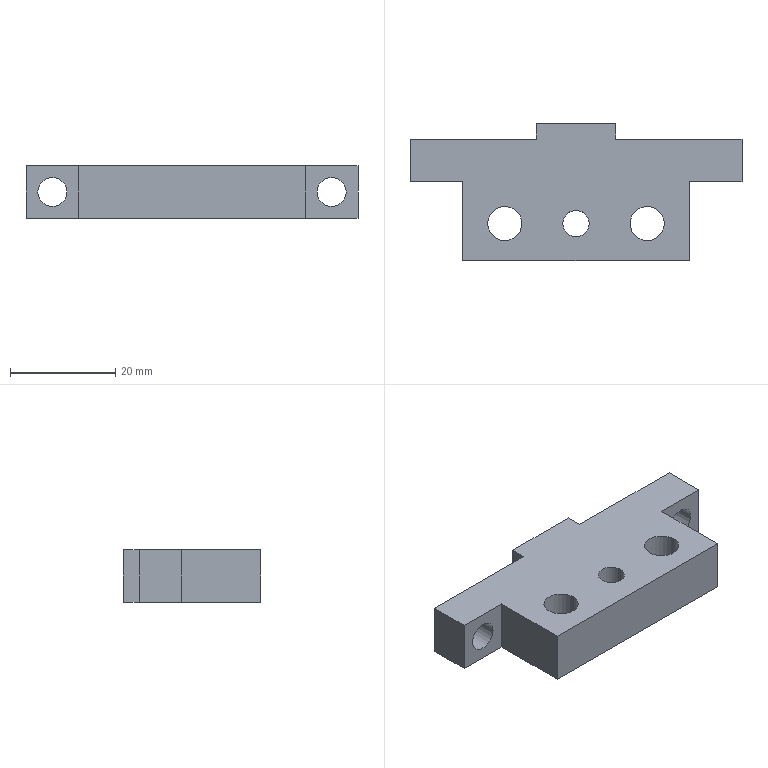Part | STEP file | Stopper buffer seat | 1 solid | 24 faces | box 63 x 26 x 10 mm | volume 10700 mm3 | plane 14 | cylinder 10 | commonest cylinder face diameters 5.5 x4 6.5 x4 5 x2